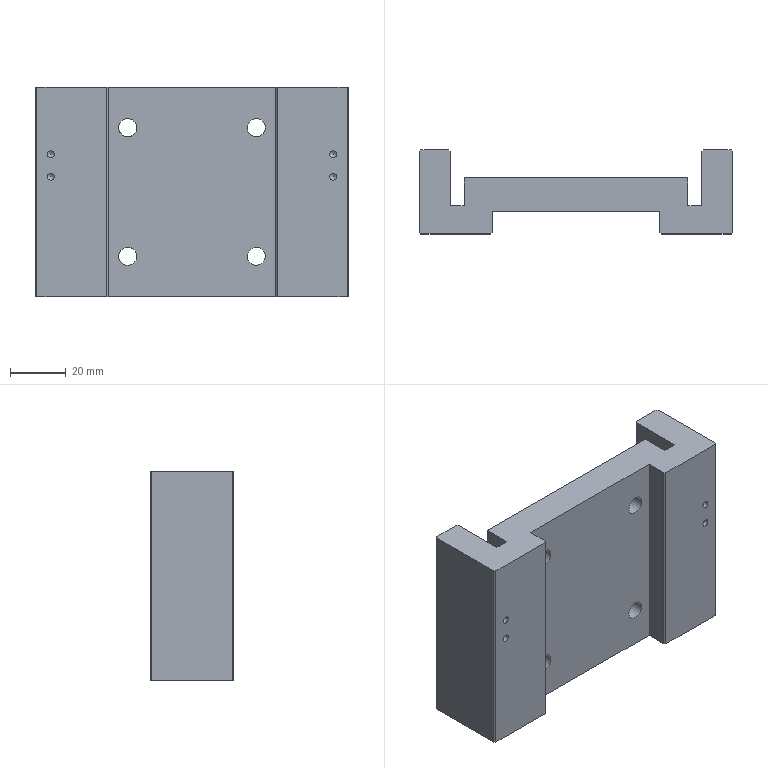Part | NX | 1 solid | 54 faces | box 112 x 30 x 75 mm | volume 135942 mm3 | plane 30 | cylinder 16 | cone 8 | commonest cylinder face diameters 2.5 x4 5 x4 6.5 x4 11 x4
STEP:
#1=CARTESIAN_POINT('',(-30.,-7.5,37.5));
#2=VERTEX_POINT('',#1);
#3=CARTESIAN_POINT('',(-30.,0.,37.5));
#4=VERTEX_POINT('',#3);
#5=CARTESIAN_POINT('',(-30.,0.,37.5));
#6=DIRECTION('',(0.,1.,0.));
#7=VECTOR('',#6,1000.);
#8=LINE('',#5,#7);
#9=EDGE_CURVE('',#2,#4,#8,.T.);
#10=ORIENTED_EDGE('',*,*,#9,.F.);
#11=CARTESIAN_POINT('',(-30.,-7.5,-37.5));
#12=VERTEX_POINT('',#11);
#13=CARTESIAN_POINT('',(-30.,-7.5,37.5));
#14=DIRECTION('',(0.,0.,-1.));
#15=VECTOR('',#14,1000.);
#16=LINE('',#13,#15);
#17=EDGE_CURVE('',#2,#12,#16,.T.);
#18=ORIENTED_EDGE('',*,*,#17,.T.);
#19=CARTESIAN_POINT('',(-30.,0.,-37.5));
#20=VERTEX_POINT('',#19);
#21=CARTESIAN_POINT('',(-30.,0.,-37.5));
#22=DIRECTION('',(0.,1.,0.));
#23=VECTOR('',#22,1000.);
#24=LINE('',#21,#23);
#25=EDGE_CURVE('',#12,#20,#24,.T.);
#26=ORIENTED_EDGE('',*,*,#25,.T.);
#27=CARTESIAN_POINT('',(-30.,0.,37.5));
#28=DIRECTION('',(0.,0.,-1.));
#29=VECTOR('',#28,1000.);
#30=LINE('',#27,#29);
#31=EDGE_CURVE('',#4,#20,#30,.T.);
#32=ORIENTED_EDGE('',*,*,#31,.F.);
#33=EDGE_LOOP('',(#10,#18,#26,#32));
#34=FACE_BOUND('',#33,.T.);
#35=CARTESIAN_POINT('',(-30.,0.,37.5));
#36=DIRECTION('',(-1.,0.,0.));
#37=DIRECTION('',(0.,-1.,0.));
#38=AXIS2_PLACEMENT_3D('',#35,#36,#37);
#39=PLANE('',#38);
#40=ADVANCED_FACE('',(#34),#39,.F.);
#41=CARTESIAN_POINT('',(-26.25,0.,-23.));
#42=VERTEX_POINT('',#41);
#43=CARTESIAN_POINT('',(-23.,0.,-23.));
#44=DIRECTION('',(0.,1.,0.));
#45=DIRECTION('',(-1.,0.,0.));
#46=AXIS2_PLACEMENT_3D('',#43,#44,#45);
#47=CIRCLE('',#46,3.25);
#48=EDGE_CURVE('',#42,#42,#47,.T.);
#49=ORIENTED_EDGE('',*,*,#48,.T.);
#50=EDGE_LOOP('',(#49));
#51=FACE_BOUND('',#50,.T.);
#52=CARTESIAN_POINT('',(-26.25,0.,23.));
#53=VERTEX_POINT('',#52);
#54=CARTESIAN_POINT('',(-23.,0.,23.));
#55=DIRECTION('',(0.,1.,0.));
#56=DIRECTION('',(-1.,0.,0.));
#57=AXIS2_PLACEMENT_3D('',#54,#55,#56);
#58=CIRCLE('',#57,3.25);
#59=EDGE_CURVE('',#53,#53,#58,.T.);
#60=ORIENTED_EDGE('',*,*,#59,.T.);
#61=EDGE_LOOP('',(#60));
#62=FACE_BOUND('',#61,.T.);
#63=CARTESIAN_POINT('',(19.75,0.,23.));
#64=VERTEX_POINT('',#63);
#65=CARTESIAN_POINT('',(23.,0.,23.));
#66=DIRECTION('',(0.,1.,0.));
#67=DIRECTION('',(-1.,0.,0.));
#68=AXIS2_PLACEMENT_3D('',#65,#66,#67);
#69=CIRCLE('',#68,3.25);
#70=EDGE_CURVE('',#64,#64,#69,.T.);
#71=ORIENTED_EDGE('',*,*,#70,.T.);
#72=EDGE_LOOP('',(#71));
#73=FACE_BOUND('',#72,.T.);
#74=CARTESIAN_POINT('',(19.75,0.,-23.));
#75=VERTEX_POINT('',#74);
#76=CARTESIAN_POINT('',(23.,0.,-23.));
#77=DIRECTION('',(0.,1.,0.));
#78=DIRECTION('',(-1.,0.,0.));
#79=AXIS2_PLACEMENT_3D('',#76,#77,#78);
#80=CIRCLE('',#79,3.25);
#81=EDGE_CURVE('',#75,#75,#80,.T.);
#82=ORIENTED_EDGE('',*,*,#81,.T.);
#83=EDGE_LOOP('',(#82));
#84=FACE_BOUND('',#83,.T.);
#85=CARTESIAN_POINT('',(30.,0.,-37.5));
#86=VERTEX_POINT('',#85);
#87=CARTESIAN_POINT('',(30.,0.,-37.5));
#88=DIRECTION('',(1.,0.,0.));
#89=VECTOR('',#88,1000.);
#90=LINE('',#87,#89);
#91=EDGE_CURVE('',#20,#86,#90,.T.);
#92=ORIENTED_EDGE('',*,*,#91,.T.);
#93=CARTESIAN_POINT('',(30.,0.,37.5));
#94=VERTEX_POINT('',#93);
#95=CARTESIAN_POINT('',(30.,0.,37.5));
#96=DIRECTION('',(0.,0.,-1.));
#97=VECTOR('',#96,1000.);
#98=LINE('',#95,#97);
#99=EDGE_CURVE('',#94,#86,#98,.T.);
#100=ORIENTED_EDGE('',*,*,#99,.F.);
#101=CARTESIAN_POINT('',(30.,0.,37.5));
#102=DIRECTION('',(1.,0.,0.));
#103=VECTOR('',#102,1000.);
#104=LINE('',#101,#103);
#105=EDGE_CURVE('',#4,#94,#104,.T.);
#106=ORIENTED_EDGE('',*,*,#105,.F.);
#107=ORIENTED_EDGE('',*,*,#31,.T.);
#108=EDGE_LOOP('',(#92,#100,#106,#107));
#109=FACE_BOUND('',#108,.T.);
#110=CARTESIAN_POINT('',(30.,0.,37.5));
#111=DIRECTION('',(0.,1.,0.));
#112=DIRECTION('',(-1.,0.,0.));
#113=AXIS2_PLACEMENT_3D('',#110,#111,#112);
#114=PLANE('',#113);
#115=ADVANCED_FACE('',(#51,#62,#73,#84,#109),#114,.F.);
#116=CARTESIAN_POINT('',(30.,-7.5,-37.5));
#117=VERTEX_POINT('',#116);
#118=CARTESIAN_POINT('',(30.,0.,-37.5));
#119=DIRECTION('',(0.,-1.,0.));
#120=VECTOR('',#119,1000.);
#121=LINE('',#118,#120);
#122=EDGE_CURVE('',#86,#117,#121,.T.);
#123=ORIENTED_EDGE('',*,*,#122,.T.);
#124=CARTESIAN_POINT('',(30.,-7.5,37.5));
#125=VERTEX_POINT('',#124);
#126=CARTESIAN_POINT('',(30.,-7.5,37.5));
#127=DIRECTION('',(0.,0.,1.));
#128=VECTOR('',#127,1000.);
#129=LINE('',#126,#128);
#130=EDGE_CURVE('',#117,#125,#129,.T.);
#131=ORIENTED_EDGE('',*,*,#130,.T.);
#132=CARTESIAN_POINT('',(30.,0.,37.5));
#133=DIRECTION('',(0.,-1.,0.));
#134=VECTOR('',#133,1000.);
#135=LINE('',#132,#134);
#136=EDGE_CURVE('',#94,#125,#135,.T.);
#137=ORIENTED_EDGE('',*,*,#136,.F.);
#138=ORIENTED_EDGE('',*,*,#99,.T.);
#139=EDGE_LOOP('',(#123,#131,#137,#138));
#140=FACE_BOUND('',#139,.T.);
#141=CARTESIAN_POINT('',(30.,0.,37.5));
#142=DIRECTION('',(1.,0.,0.));
#143=DIRECTION('',(0.,0.,-1.));
#144=AXIS2_PLACEMENT_3D('',#141,#142,#143);
#145=PLANE('',#144);
#146=ADVANCED_FACE('',(#140),#145,.F.);
#147=CARTESIAN_POINT('',(50.5,-8.,12.25));
#148=VERTEX_POINT('',#147);
#149=CARTESIAN_POINT('',(50.5,-8.,13.5));
#150=DIRECTION('',(0.,-1.,0.));
#151=DIRECTION('',(0.,0.,-1.));
#152=AXIS2_PLACEMENT_3D('',#149,#150,#151);
#153=CIRCLE('',#152,1.25);
#154=EDGE_CURVE('',#148,#148,#153,.T.);
#155=ORIENTED_EDGE('',*,*,#154,.F.);
#156=EDGE_LOOP('',(#155));
#157=FACE_BOUND('',#156,.T.);
#158=CARTESIAN_POINT('',(50.5,-8.,4.25));
#159=VERTEX_POINT('',#158);
#160=CARTESIAN_POINT('',(50.5,-8.,5.5));
#161=DIRECTION('',(0.,-1.,0.));
#162=DIRECTION('',(0.,0.,-1.));
#163=AXIS2_PLACEMENT_3D('',#160,#161,#162);
#164=CIRCLE('',#163,1.25);
#165=EDGE_CURVE('',#159,#159,#164,.T.);
#166=ORIENTED_EDGE('',*,*,#165,.F.);
#167=EDGE_LOOP('',(#166));
#168=FACE_BOUND('',#167,.T.);
#169=CARTESIAN_POINT('',(30.5,-8.,-37.5));
#170=VERTEX_POINT('',#169);
#171=CARTESIAN_POINT('',(55.5,-8.,-37.5));
#172=VERTEX_POINT('',#171);
#173=CARTESIAN_POINT('',(30.,-8.,-37.5));
#174=DIRECTION('',(1.,0.,0.));
#175=VECTOR('',#174,1000.);
#176=LINE('',#173,#175);
#177=EDGE_CURVE('',#170,#172,#176,.T.);
#178=ORIENTED_EDGE('',*,*,#177,.T.);
#179=CARTESIAN_POINT('',(55.5,-8.,37.5));
#180=VERTEX_POINT('',#179);
#181=CARTESIAN_POINT('',(55.5,-8.,37.5));
#182=DIRECTION('',(0.,0.,1.));
#183=VECTOR('',#182,1000.);
#184=LINE('',#181,#183);
#185=EDGE_CURVE('',#172,#180,#184,.T.);
#186=ORIENTED_EDGE('',*,*,#185,.T.);
#187=CARTESIAN_POINT('',(30.5,-8.,37.5));
#188=VERTEX_POINT('',#187);
#189=CARTESIAN_POINT('',(30.,-8.,37.5));
#190=DIRECTION('',(1.,0.,0.));
#191=VECTOR('',#190,1000.);
#192=LINE('',#189,#191);
#193=EDGE_CURVE('',#188,#180,#192,.T.);
#194=ORIENTED_EDGE('',*,*,#193,.F.);
#195=CARTESIAN_POINT('',(30.5,-8.,37.5));
#196=DIRECTION('',(0.,0.,-1.));
#197=VECTOR('',#196,1000.);
#198=LINE('',#195,#197);
#199=EDGE_CURVE('',#188,#170,#198,.T.);
#200=ORIENTED_EDGE('',*,*,#199,.T.);
#201=EDGE_LOOP('',(#178,#186,#194,#200));
#202=FACE_BOUND('',#201,.T.);
#203=CARTESIAN_POINT('',(30.,-8.,37.5));
#204=DIRECTION('',(0.,1.,0.));
#205=DIRECTION('',(-1.,0.,0.));
#206=AXIS2_PLACEMENT_3D('',#203,#204,#205);
#207=PLANE('',#206);
#208=ADVANCED_FACE('',(#157,#168,#202),#207,.F.);
#209=CARTESIAN_POINT('',(56.,-7.5,-37.5));
#210=VERTEX_POINT('',#209);
#211=CARTESIAN_POINT('',(56.,21.5,-37.5));
#212=VERTEX_POINT('',#211);
#213=CARTESIAN_POINT('',(56.,-8.,-37.5));
#214=DIRECTION('',(0.,1.,0.));
#215=VECTOR('',#214,1000.);
#216=LINE('',#213,#215);
#217=EDGE_CURVE('',#210,#212,#216,.T.);
#218=ORIENTED_EDGE('',*,*,#217,.T.);
#219=CARTESIAN_POINT('',(56.,21.5,37.5));
#220=VERTEX_POINT('',#219);
#221=CARTESIAN_POINT('',(56.,21.5,37.5));
#222=DIRECTION('',(0.,0.,1.));
#223=VECTOR('',#222,1000.);
#224=LINE('',#221,#223);
#225=EDGE_CURVE('',#212,#220,#224,.T.);
#226=ORIENTED_EDGE('',*,*,#225,.T.);
#227=CARTESIAN_POINT('',(56.,-7.5,37.5));
#228=VERTEX_POINT('',#227);
#229=CARTESIAN_POINT('',(56.,-8.,37.5));
#230=DIRECTION('',(0.,1.,0.));
#231=VECTOR('',#230,1000.);
#232=LINE('',#229,#231);
#233=EDGE_CURVE('',#228,#220,#232,.T.);
#234=ORIENTED_EDGE('',*,*,#233,.F.);
#235=CARTESIAN_POINT('',(56.,-7.5,37.5));
#236=DIRECTION('',(0.,0.,-1.));
#237=VECTOR('',#236,1000.);
#238=LINE('',#235,#237);
#239=EDGE_CURVE('',#228,#210,#238,.T.);
#240=ORIENTED_EDGE('',*,*,#239,.T.);
#241=EDGE_LOOP('',(#218,#226,#234,#240));
#242=FACE_BOUND('',#241,.T.);
#243=CARTESIAN_POINT('',(56.,-8.,37.5));
#244=DIRECTION('',(-1.,0.,0.));
#245=DIRECTION('',(0.,-1.,0.));
#246=AXIS2_PLACEMENT_3D('',#243,#244,#245);
#247=PLANE('',#246);
#248=ADVANCED_FACE('',(#242),#247,.F.);
#249=CARTESIAN_POINT('',(50.,22.,-20.5));
#250=VERTEX_POINT('',#249);
#251=CARTESIAN_POINT('',(50.,22.,-23.));
#252=DIRECTION('',(0.,1.,0.));
#253=DIRECTION('',(0.,0.,1.));
#254=AXIS2_PLACEMENT_3D('',#251,#252,#253);
#255=CIRCLE('',#254,2.5);
#256=EDGE_CURVE('',#250,#250,#255,.T.);
#257=ORIENTED_EDGE('',*,*,#256,.F.);
#258=EDGE_LOOP('',(#257));
#259=FACE_BOUND('',#258,.T.);
#260=CARTESIAN_POINT('',(50.,22.,25.5));
#261=VERTEX_POINT('',#260);
#262=CARTESIAN_POINT('',(50.,22.,23.));
#263=DIRECTION('',(0.,1.,0.));
#264=DIRECTION('',(0.,0.,1.));
#265=AXIS2_PLACEMENT_3D('',#262,#263,#264);
#266=CIRCLE('',#265,2.5);
#267=EDGE_CURVE('',#261,#261,#266,.T.);
#268=ORIENTED_EDGE('',*,*,#267,.F.);
#269=EDGE_LOOP('',(#268));
#270=FACE_BOUND('',#269,.T.);
#271=CARTESIAN_POINT('',(55.5,22.,-37.5));
#272=VERTEX_POINT('',#271);
#273=CARTESIAN_POINT('',(45.5,22.,-37.5));
#274=VERTEX_POINT('',#273);
#275=CARTESIAN_POINT('',(56.,22.,-37.5));
#276=DIRECTION('',(-1.,0.,0.));
#277=VECTOR('',#276,1000.);
#278=LINE('',#275,#277);
#279=EDGE_CURVE('',#272,#274,#278,.T.);
#280=ORIENTED_EDGE('',*,*,#279,.T.);
#281=CARTESIAN_POINT('',(45.5,22.,37.5));
#282=VERTEX_POINT('',#281);
#283=CARTESIAN_POINT('',(45.5,22.,37.5));
#284=DIRECTION('',(0.,0.,1.));
#285=VECTOR('',#284,1000.);
#286=LINE('',#283,#285);
#287=EDGE_CURVE('',#274,#282,#286,.T.);
#288=ORIENTED_EDGE('',*,*,#287,.T.);
#289=CARTESIAN_POINT('',(55.5,22.,37.5));
#290=VERTEX_POINT('',#289);
#291=CARTESIAN_POINT('',(56.,22.,37.5));
#292=DIRECTION('',(-1.,0.,0.));
#293=VECTOR('',#292,1000.);
#294=LINE('',#291,#293);
#295=EDGE_CURVE('',#290,#282,#294,.T.);
#296=ORIENTED_EDGE('',*,*,#295,.F.);
#297=CARTESIAN_POINT('',(55.5,22.,37.5));
#298=DIRECTION('',(0.,0.,-1.));
#299=VECTOR('',#298,1000.);
#300=LINE('',#297,#299);
#301=EDGE_CURVE('',#290,#272,#300,.T.);
#302=ORIENTED_EDGE('',*,*,#301,.T.);
#303=EDGE_LOOP('',(#280,#288,#296,#302));
#304=FACE_BOUND('',#303,.T.);
#305=CARTESIAN_POINT('',(56.,22.,37.5));
#306=DIRECTION('',(0.,-1.,0.));
#307=DIRECTION('',(0.,0.,-1.));
#308=AXIS2_PLACEMENT_3D('',#305,#306,#307);
#309=PLANE('',#308);
#310=ADVANCED_FACE('',(#259,#270,#304),#309,.F.);
#311=CARTESIAN_POINT('',(45.,21.5,37.5));
#312=VERTEX_POINT('',#311);
#313=CARTESIAN_POINT('',(45.,2.,37.5));
#314=VERTEX_POINT('',#313);
#315=CARTESIAN_POINT('',(45.,22.,37.5));
#316=DIRECTION('',(0.,-1.,0.));
#317=VECTOR('',#316,1000.);
#318=LINE('',#315,#317);
#319=EDGE_CURVE('',#312,#314,#318,.T.);
#320=ORIENTED_EDGE('',*,*,#319,.F.);
#321=CARTESIAN_POINT('',(45.,21.5,-37.5));
#322=VERTEX_POINT('',#321);
#323=CARTESIAN_POINT('',(45.,21.5,37.5));
#324=DIRECTION('',(0.,0.,-1.));
#325=VECTOR('',#324,1000.);
#326=LINE('',#323,#325);
#327=EDGE_CURVE('',#312,#322,#326,.T.);
#328=ORIENTED_EDGE('',*,*,#327,.T.);
#329=CARTESIAN_POINT('',(45.,2.,-37.5));
#330=VERTEX_POINT('',#329);
#331=CARTESIAN_POINT('',(45.,22.,-37.5));
#332=DIRECTION('',(0.,-1.,0.));
#333=VECTOR('',#332,1000.);
#334=LINE('',#331,#333);
#335=EDGE_CURVE('',#322,#330,#334,.T.);
#336=ORIENTED_EDGE('',*,*,#335,.T.);
#337=CARTESIAN_POINT('',(45.,2.,37.5));
#338=DIRECTION('',(0.,0.,-1.));
#339=VECTOR('',#338,1000.);
#340=LINE('',#337,#339);
#341=EDGE_CURVE('',#314,#330,#340,.T.);
#342=ORIENTED_EDGE('',*,*,#341,.F.);
#343=EDGE_LOOP('',(#320,#328,#336,#342));
#344=FACE_BOUND('',#343,.T.);
#345=CARTESIAN_POINT('',(45.,22.,37.5));
#346=DIRECTION('',(1.,0.,0.));
#347=DIRECTION('',(0.,0.,-1.));
#348=AXIS2_PLACEMENT_3D('',#345,#346,#347);
#349=PLANE('',#348);
#350=ADVANCED_FACE('',(#344),#349,.F.);
#351=CARTESIAN_POINT('',(-23.,12.,-17.5));
#352=VERTEX_POINT('',#351);
#353=CARTESIAN_POINT('',(-23.,12.,-23.));
#354=DIRECTION('',(0.,1.,0.));
#355=DIRECTION('',(0.,0.,1.));
#356=AXIS2_PLACEMENT_3D('',#353,#354,#355);
#357=CIRCLE('',#356,5.5);
#358=EDGE_CURVE('',#352,#352,#357,.T.);
#359=ORIENTED_EDGE('',*,*,#358,.F.);
#360=EDGE_LOOP('',(#359));
#361=FACE_BOUND('',#360,.T.);
#362=CARTESIAN_POINT('',(-23.,12.,28.5));
#363=VERTEX_POINT('',#362);
#364=CARTESIAN_POINT('',(-23.,12.,23.));
#365=DIRECTION('',(0.,1.,0.));
#366=DIRECTION('',(0.,0.,1.));
#367=AXIS2_PLACEMENT_3D('',#364,#365,#366);
#368=CIRCLE('',#367,5.5);
#369=EDGE_CURVE('',#363,#363,#368,.T.);
#370=ORIENTED_EDGE('',*,*,#369,.F.);
#371=EDGE_LOOP('',(#370));
#372=FACE_BOUND('',#371,.T.);
#373=CARTESIAN_POINT('',(23.,12.,28.5));
#374=VERTEX_POINT('',#373);
#375=CARTESIAN_POINT('',(23.,12.,23.));
#376=DIRECTION('',(0.,1.,0.));
#377=DIRECTION('',(0.,0.,1.));
#378=AXIS2_PLACEMENT_3D('',#375,#376,#377);
#379=CIRCLE('',#378,5.5);
#380=EDGE_CURVE('',#374,#374,#379,.T.);
#381=ORIENTED_EDGE('',*,*,#380,.F.);
#382=EDGE_LOOP('',(#381));
#383=FACE_BOUND('',#382,.T.);
#384=CARTESIAN_POINT('',(23.,12.,-17.5));
#385=VERTEX_POINT('',#384);
#386=CARTESIAN_POINT('',(23.,12.,-23.));
#387=DIRECTION('',(0.,1.,0.));
#388=DIRECTION('',(0.,0.,1.));
#389=AXIS2_PLACEMENT_3D('',#386,#387,#388);
#390=CIRCLE('',#389,5.5);
#391=EDGE_CURVE('',#385,#385,#390,.T.);
#392=ORIENTED_EDGE('',*,*,#391,.F.);
#393=EDGE_LOOP('',(#392));
#394=FACE_BOUND('',#393,.T.);
#395=CARTESIAN_POINT('',(40.,12.,-37.5));
#396=VERTEX_POINT('',#395);
#397=CARTESIAN_POINT('',(-40.,12.,-37.5));
#398=VERTEX_POINT('',#397);
#399=CARTESIAN_POINT('',(-45.,12.,-37.5));
#400=DIRECTION('',(-1.,0.,0.));
#401=VECTOR('',#400,1000.);
#402=LINE('',#399,#401);
#403=EDGE_CURVE('',#396,#398,#402,.T.);
#404=ORIENTED_EDGE('',*,*,#403,.T.);
#405=CARTESIAN_POINT('',(-40.,12.,37.5));
#406=VERTEX_POINT('',#405);
#407=CARTESIAN_POINT('',(-40.,12.,37.5));
#408=DIRECTION('',(0.,0.,-1.));
#409=VECTOR('',#408,1000.);
#410=LINE('',#407,#409);
#411=EDGE_CURVE('',#406,#398,#410,.T.);
#412=ORIENTED_EDGE('',*,*,#411,.F.);
#413=CARTESIAN_POINT('',(40.,12.,37.5));
#414=VERTEX_POINT('',#413);
#415=CARTESIAN_POINT('',(-45.,12.,37.5));
#416=DIRECTION('',(-1.,0.,0.));
#417=VECTOR('',#416,1000.);
#418=LINE('',#415,#417);
#419=EDGE_CURVE('',#414,#406,#418,.T.);
#420=ORIENTED_EDGE('',*,*,#419,.F.);
#421=CARTESIAN_POINT('',(40.,12.,37.5));
#422=DIRECTION('',(0.,0.,-1.));
#423=VECTOR('',#422,1000.);
#424=LINE('',#421,#423);
#425=EDGE_CURVE('',#414,#396,#424,.T.);
#426=ORIENTED_EDGE('',*,*,#425,.T.);
#427=EDGE_LOOP('',(#404,#412,#420,#426));
#428=FACE_BOUND('',#427,.T.);
#429=CARTESIAN_POINT('',(-45.,12.,37.5));
#430=DIRECTION('',(0.,-1.,0.));
#431=DIRECTION('',(1.,0.,0.));
#432=AXIS2_PLACEMENT_3D('',#429,#430,#431);
#433=PLANE('',#432);
#434=ADVANCED_FACE('',(#361,#372,#383,#394,#428),#433,.F.);
#435=CARTESIAN_POINT('',(-45.,2.,-37.5));
#436=VERTEX_POINT('',#435);
#437=CARTESIAN_POINT('',(-45.,21.5,-37.5));
#438=VERTEX_POINT('',#437);
#439=CARTESIAN_POINT('',(-45.,22.,-37.5));
#440=DIRECTION('',(0.,1.,0.));
#441=VECTOR('',#440,1000.);
#442=LINE('',#439,#441);
#443=EDGE_CURVE('',#436,#438,#442,.T.);
#444=ORIENTED_EDGE('',*,*,#443,.T.);
#445=CARTESIAN_POINT('',(-45.,21.5,37.5));
#446=VERTEX_POINT('',#445);
#447=CARTESIAN_POINT('',(-45.,21.5,37.5));
#448=DIRECTION('',(0.,0.,1.));
#449=VECTOR('',#448,1000.);
#450=LINE('',#447,#449);
#451=EDGE_CURVE('',#438,#446,#450,.T.);
#452=ORIENTED_EDGE('',*,*,#451,.T.);
#453=CARTESIAN_POINT('',(-45.,2.,37.5));
#454=VERTEX_POINT('',#453);
#455=CARTESIAN_POINT('',(-45.,22.,37.5));
#456=DIRECTION('',(0.,1.,0.));
#457=VECTOR('',#456,1000.);
#458=LINE('',#455,#457);
#459=EDGE_CURVE('',#454,#446,#458,.T.);
#460=ORIENTED_EDGE('',*,*,#459,.F.);
#461=CARTESIAN_POINT('',(-45.,2.,37.5));
#462=DIRECTION('',(0.,0.,-1.));
#463=VECTOR('',#462,1000.);
#464=LINE('',#461,#463);
#465=EDGE_CURVE('',#454,#436,#464,.T.);
#466=ORIENTED_EDGE('',*,*,#465,.T.);
#467=EDGE_LOOP('',(#444,#452,#460,#466));
#468=FACE_BOUND('',#467,.T.);
#469=CARTESIAN_POINT('',(-45.,22.,37.5));
#470=DIRECTION('',(-1.,0.,0.));
#471=DIRECTION('',(0.,0.,1.));
#472=AXIS2_PLACEMENT_3D('',#469,#470,#471);
#473=PLANE('',#472);
#474=ADVANCED_FACE('',(#468),#473,.F.);
#475=CARTESIAN_POINT('',(-50.,22.,-20.5));
#476=VERTEX_POINT('',#475);
#477=CARTESIAN_POINT('',(-50.,22.,-23.));
#478=DIRECTION('',(0.,1.,0.));
#479=DIRECTION('',(0.,0.,1.));
#480=AXIS2_PLACEMENT_3D('',#477,#478,#479);
#481=CIRCLE('',#480,2.5);
#482=EDGE_CURVE('',#476,#476,#481,.T.);
#483=ORIENTED_EDGE('',*,*,#482,.F.);
#484=EDGE_LOOP('',(#483));
#485=FACE_BOUND('',#484,.T.);
#486=CARTESIAN_POINT('',(-50.,22.,25.5));
#487=VERTEX_POINT('',#486);
#488=CARTESIAN_POINT('',(-50.,22.,23.));
#489=DIRECTION('',(0.,1.,0.));
#490=DIRECTION('',(0.,0.,1.));
#491=AXIS2_PLACEMENT_3D('',#488,#489,#490);
#492=CIRCLE('',#491,2.5);
#493=EDGE_CURVE('',#487,#487,#492,.T.);
#494=ORIENTED_EDGE('',*,*,#493,.F.);
#495=EDGE_LOOP('',(#494));
#496=FACE_BOUND('',#495,.T.);
#497=CARTESIAN_POINT('',(-45.5,22.,-37.5));
#498=VERTEX_POINT('',#497);
#499=CARTESIAN_POINT('',(-55.5,22.,-37.5));
#500=VERTEX_POINT('',#499);
#501=CARTESIAN_POINT('',(-56.,22.,-37.5));
#502=DIRECTION('',(-1.,0.,0.));
#503=VECTOR('',#502,1000.);
#504=LINE('',#501,#503);
#505=EDGE_CURVE('',#498,#500,#504,.T.);
#506=ORIENTED_EDGE('',*,*,#505,.T.);
#507=CARTESIAN_POINT('',(-55.5,22.,37.5));
#508=VERTEX_POINT('',#507);
#509=CARTESIAN_POINT('',(-55.5,22.,37.5));
#510=DIRECTION('',(0.,0.,1.));
#511=VECTOR('',#510,1000.);
#512=LINE('',#509,#511);
#513=EDGE_CURVE('',#500,#508,#512,.T.);
#514=ORIENTED_EDGE('',*,*,#513,.T.);
#515=CARTESIAN_POINT('',(-45.5,22.,37.5));
#516=VERTEX_POINT('',#515);
#517=CARTESIAN_POINT('',(-56.,22.,37.5));
#518=DIRECTION('',(-1.,0.,0.));
#519=VECTOR('',#518,1000.);
#520=LINE('',#517,#519);
#521=EDGE_CURVE('',#516,#508,#520,.T.);
#522=ORIENTED_EDGE('',*,*,#521,.F.);
#523=CARTESIAN_POINT('',(-45.5,22.,37.5));
#524=DIRECTION('',(0.,0.,-1.));
#525=VECTOR('',#524,1000.);
#526=LINE('',#523,#525);
#527=EDGE_CURVE('',#516,#498,#526,.T.);
#528=ORIENTED_EDGE('',*,*,#527,.T.);
#529=EDGE_LOOP('',(#506,#514,#522,#528));
#530=FACE_BOUND('',#529,.T.);
#531=CARTESIAN_POINT('',(-56.,22.,37.5));
#532=DIRECTION('',(0.,-1.,0.));
#533=DIRECTION('',(1.,0.,0.));
#534=AXIS2_PLACEMENT_3D('',#531,#532,#533);
#535=PLANE('',#534);
#536=ADVANCED_FACE('',(#485,#496,#530),#535,.F.);
#537=CARTESIAN_POINT('',(-56.,21.5,37.5));
#538=VERTEX_POINT('',#537);
#539=CARTESIAN_POINT('',(-56.,-7.5,37.5));
#540=VERTEX_POINT('',#539);
#541=CARTESIAN_POINT('',(-56.,-8.,37.5));
#542=DIRECTION('',(0.,-1.,0.));
#543=VECTOR('',#542,1000.);
#544=LINE('',#541,#543);
#545=EDGE_CURVE('',#538,#540,#544,.T.);
#546=ORIENTED_EDGE('',*,*,#545,.F.);
#547=CARTESIAN_POINT('',(-56.,21.5,-37.5));
#548=VERTEX_POINT('',#547);
#549=CARTESIAN_POINT('',(-56.,21.5,37.5));
#550=DIRECTION('',(0.,0.,-1.));
#551=VECTOR('',#550,1000.);
#552=LINE('',#549,#551);
#553=EDGE_CURVE('',#538,#548,#552,.T.);
#554=ORIENTED_EDGE('',*,*,#553,.T.);
#555=CARTESIAN_POINT('',(-56.,-7.5,-37.5));
#556=VERTEX_POINT('',#555);
#557=CARTESIAN_POINT('',(-56.,-8.,-37.5));
#558=DIRECTION('',(0.,-1.,0.));
#559=VECTOR('',#558,1000.);
#560=LINE('',#557,#559);
#561=EDGE_CURVE('',#548,#556,#560,.T.);
#562=ORIENTED_EDGE('',*,*,#561,.T.);
#563=CARTESIAN_POINT('',(-56.,-7.5,37.5));
#564=DIRECTION('',(0.,0.,1.));
#565=VECTOR('',#564,1000.);
#566=LINE('',#563,#565);
#567=EDGE_CURVE('',#556,#540,#566,.T.);
#568=ORIENTED_EDGE('',*,*,#567,.T.);
#569=EDGE_LOOP('',(#546,#554,#562,#568));
#570=FACE_BOUND('',#569,.T.);
#571=CARTESIAN_POINT('',(-56.,-8.,37.5));
#572=DIRECTION('',(1.,0.,0.));
#573=DIRECTION('',(0.,1.,0.));
#574=AXIS2_PLACEMENT_3D('',#571,#572,#573);
#575=PLANE('',#574);
#576=ADVANCED_FACE('',(#570),#575,.F.);
#577=CARTESIAN_POINT('',(-50.5,-8.,12.25));
#578=VERTEX_POINT('',#577);
#579=CARTESIAN_POINT('',(-50.5,-8.,13.5));
#580=DIRECTION('',(0.,-1.,0.));
#581=DIRECTION('',(0.,0.,-1.));
#582=AXIS2_PLACEMENT_3D('',#579,#580,#581);
#583=CIRCLE('',#582,1.25);
#584=EDGE_CURVE('',#578,#578,#583,.T.);
#585=ORIENTED_EDGE('',*,*,#584,.F.);
#586=EDGE_LOOP('',(#585));
#587=FACE_BOUND('',#586,.T.);
#588=CARTESIAN_POINT('',(-50.5,-8.,4.25));
#589=VERTEX_POINT('',#588);
#590=CARTESIAN_POINT('',(-50.5,-8.,5.5));
#591=DIRECTION('',(0.,-1.,0.));
#592=DIRECTION('',(0.,0.,-1.));
#593=AXIS2_PLACEMENT_3D('',#590,#591,#592);
#594=CIRCLE('',#593,1.25);
#595=EDGE_CURVE('',#589,#589,#594,.T.);
#596=ORIENTED_EDGE('',*,*,#595,.F.);
#597=EDGE_LOOP('',(#596));
#598=FACE_BOUND('',#597,.T.);
#599=CARTESIAN_POINT('',(-55.5,-8.,-37.5));
#600=VERTEX_POINT('',#599);
#601=CARTESIAN_POINT('',(-30.5,-8.,-37.5));
#602=VERTEX_POINT('',#601);
#603=CARTESIAN_POINT('',(-30.,-8.,-37.5));
#604=DIRECTION('',(1.,0.,0.));
#605=VECTOR('',#604,1000.);
#606=LINE('',#603,#605);
#607=EDGE_CURVE('',#600,#602,#606,.T.);
#608=ORIENTED_EDGE('',*,*,#607,.T.);
#609=CARTESIAN_POINT('',(-30.5,-8.,37.5));
#610=VERTEX_POINT('',#609);
#611=CARTESIAN_POINT('',(-30.5,-8.,37.5));
#612=DIRECTION('',(0.,0.,1.));
#613=VECTOR('',#612,1000.);
#614=LINE('',#611,#613);
#615=EDGE_CURVE('',#602,#610,#614,.T.);
#616=ORIENTED_EDGE('',*,*,#615,.T.);
#617=CARTESIAN_POINT('',(-55.5,-8.,37.5));
#618=VERTEX_POINT('',#617);
#619=CARTESIAN_POINT('',(-30.,-8.,37.5));
#620=DIRECTION('',(1.,0.,0.));
#621=VECTOR('',#620,1000.);
#622=LINE('',#619,#621);
#623=EDGE_CURVE('',#618,#610,#622,.T.);
#624=ORIENTED_EDGE('',*,*,#623,.F.);
#625=CARTESIAN_POINT('',(-55.5,-8.,37.5));
#626=DIRECTION('',(0.,0.,-1.));
#627=VECTOR('',#626,1000.);
#628=LINE('',#625,#627);
#629=EDGE_CURVE('',#618,#600,#628,.T.);
#630=ORIENTED_EDGE('',*,*,#629,.T.);
#631=EDGE_LOOP('',(#608,#616,#624,#630));
#632=FACE_BOUND('',#631,.T.);
#633=CARTESIAN_POINT('',(-30.,-8.,37.5));
#634=DIRECTION('',(0.,1.,0.));
#635=DIRECTION('',(-1.,0.,0.));
#636=AXIS2_PLACEMENT_3D('',#633,#634,#635);
#637=PLANE('',#636);
#638=ADVANCED_FACE('',(#587,#598,#632),#637,.F.);
#639=CARTESIAN_POINT('',(-40.,2.,37.5));
#640=VERTEX_POINT('',#639);
#641=CARTESIAN_POINT('',(-45.,2.,37.5));
#642=DIRECTION('',(-1.,0.,0.));
#643=VECTOR('',#642,1000.);
#644=LINE('',#641,#643);
#645=EDGE_CURVE('',#640,#454,#644,.T.);
#646=ORIENTED_EDGE('',*,*,#645,.T.);
#647=ORIENTED_EDGE('',*,*,#459,.T.);
#648=CARTESIAN_POINT('',(-45.5,22.,37.5));
#649=DIRECTION('',(0.7071,-0.7071,0.));
#650=VECTOR('',#649,1000.);
#651=LINE('',#648,#650);
#652=EDGE_CURVE('',#446,#516,#651,.F.);
#653=ORIENTED_EDGE('',*,*,#652,.T.);
#654=ORIENTED_EDGE('',*,*,#521,.T.);
#655=CARTESIAN_POINT('',(-56.,21.5,37.5));
#656=DIRECTION('',(0.7071,0.7071,0.));
#657=VECTOR('',#656,1000.);
#658=LINE('',#655,#657);
#659=EDGE_CURVE('',#508,#538,#658,.F.);
#660=ORIENTED_EDGE('',*,*,#659,.T.);
#661=ORIENTED_EDGE('',*,*,#545,.T.);
#662=CARTESIAN_POINT('',(-55.5,-8.,37.5));
#663=DIRECTION('',(-0.7071,0.7071,0.));
#664=VECTOR('',#663,1000.);
#665=LINE('',#662,#664);
#666=EDGE_CURVE('',#540,#618,#665,.F.);
#667=ORIENTED_EDGE('',*,*,#666,.T.);
#668=ORIENTED_EDGE('',*,*,#623,.T.);
#669=CARTESIAN_POINT('',(-30.,-7.5,37.5));
#670=DIRECTION('',(-0.7071,-0.7071,0.));
#671=VECTOR('',#670,1000.);
#672=LINE('',#669,#671);
#673=EDGE_CURVE('',#610,#2,#672,.F.);
#674=ORIENTED_EDGE('',*,*,#673,.T.);
#675=ORIENTED_EDGE('',*,*,#9,.T.);
#676=ORIENTED_EDGE('',*,*,#105,.T.);
#677=ORIENTED_EDGE('',*,*,#136,.T.);
#678=CARTESIAN_POINT('',(30.5,-8.,37.5));
#679=DIRECTION('',(-0.7071,0.7071,0.));
#680=VECTOR('',#679,1000.);
#681=LINE('',#678,#680);
#682=EDGE_CURVE('',#125,#188,#681,.F.);
#683=ORIENTED_EDGE('',*,*,#682,.T.);
#684=ORIENTED_EDGE('',*,*,#193,.T.);
#685=CARTESIAN_POINT('',(56.,-7.5,37.5));
#686=DIRECTION('',(-0.7071,-0.7071,0.));
#687=VECTOR('',#686,1000.);
#688=LINE('',#685,#687);
#689=EDGE_CURVE('',#180,#228,#688,.F.);
#690=ORIENTED_EDGE('',*,*,#689,.T.);
#691=ORIENTED_EDGE('',*,*,#233,.T.);
#692=CARTESIAN_POINT('',(55.5,22.,37.5));
#693=DIRECTION('',(0.7071,-0.7071,0.));
#694=VECTOR('',#693,1000.);
#695=LINE('',#692,#694);
#696=EDGE_CURVE('',#220,#290,#695,.F.);
#697=ORIENTED_EDGE('',*,*,#696,.T.);
#698=ORIENTED_EDGE('',*,*,#295,.T.);
#699=CARTESIAN_POINT('',(45.,21.5,37.5));
#700=DIRECTION('',(0.7071,0.7071,0.));
#701=VECTOR('',#700,1000.);
#702=LINE('',#699,#701);
#703=EDGE_CURVE('',#282,#312,#702,.F.);
#704=ORIENTED_EDGE('',*,*,#703,.T.);
#705=ORIENTED_EDGE('',*,*,#319,.T.);
#706=CARTESIAN_POINT('',(40.,2.,37.5));
#707=VERTEX_POINT('',#706);
#708=CARTESIAN_POINT('',(45.,2.,37.5));
#709=DIRECTION('',(-1.,0.,0.));
#710=VECTOR('',#709,1000.);
#711=LINE('',#708,#710);
#712=EDGE_CURVE('',#314,#707,#711,.T.);
#713=ORIENTED_EDGE('',*,*,#712,.T.);
#714=CARTESIAN_POINT('',(40.,12.,37.5));
#715=DIRECTION('',(0.,1.,0.));
#716=VECTOR('',#715,1000.);
#717=LINE('',#714,#716);
#718=EDGE_CURVE('',#707,#414,#717,.T.);
#719=ORIENTED_EDGE('',*,*,#718,.T.);
#720=ORIENTED_EDGE('',*,*,#419,.T.);
#721=CARTESIAN_POINT('',(-40.,12.,37.5));
#722=DIRECTION('',(0.,-1.,0.));
#723=VECTOR('',#722,1000.);
#724=LINE('',#721,#723);
#725=EDGE_CURVE('',#406,#640,#724,.T.);
#726=ORIENTED_EDGE('',*,*,#725,.T.);
#727=EDGE_LOOP('',(#646,#647,#653,#654,#660,#661,#667,#668,#674,#675,#676,#677,#683,#684,#690,#691,#697,#698,#704,#705,#713,#719,#720,#726));
#728=FACE_BOUND('',#727,.T.);
#729=CARTESIAN_POINT('',(0.,0.,37.5));
#730=DIRECTION('',(0.,0.,-1.));
#731=DIRECTION('',(-1.,0.,0.));
#732=AXIS2_PLACEMENT_3D('',#729,#730,#731);
#733=PLANE('',#732);
#734=ADVANCED_FACE('',(#728),#733,.F.);
#735=ORIENTED_EDGE('',*,*,#443,.F.);
#736=CARTESIAN_POINT('',(-40.,2.,-37.5));
#737=VERTEX_POINT('',#736);
#738=CARTESIAN_POINT('',(-45.,2.,-37.5));
#739=DIRECTION('',(-1.,0.,0.));
#740=VECTOR('',#739,1000.);
#741=LINE('',#738,#740);
#742=EDGE_CURVE('',#737,#436,#741,.T.);
#743=ORIENTED_EDGE('',*,*,#742,.F.);
#744=CARTESIAN_POINT('',(-40.,12.,-37.5));
#745=DIRECTION('',(0.,-1.,0.));
#746=VECTOR('',#745,1000.);
#747=LINE('',#744,#746);
#748=EDGE_CURVE('',#398,#737,#747,.T.);
#749=ORIENTED_EDGE('',*,*,#748,.F.);
#750=ORIENTED_EDGE('',*,*,#403,.F.);
#751=CARTESIAN_POINT('',(40.,2.,-37.5));
#752=VERTEX_POINT('',#751);
#753=CARTESIAN_POINT('',(40.,12.,-37.5));
#754=DIRECTION('',(0.,1.,0.));
#755=VECTOR('',#754,1000.);
#756=LINE('',#753,#755);
#757=EDGE_CURVE('',#752,#396,#756,.T.);
#758=ORIENTED_EDGE('',*,*,#757,.F.);
#759=CARTESIAN_POINT('',(45.,2.,-37.5));
#760=DIRECTION('',(-1.,0.,0.));
#761=VECTOR('',#760,1000.);
#762=LINE('',#759,#761);
#763=EDGE_CURVE('',#330,#752,#762,.T.);
#764=ORIENTED_EDGE('',*,*,#763,.F.);
#765=ORIENTED_EDGE('',*,*,#335,.F.);
#766=CARTESIAN_POINT('',(11.75,-11.75,-37.5));
#767=DIRECTION('',(-0.7071,-0.7071,0.));
#768=VECTOR('',#767,1000.);
#769=LINE('',#766,#768);
#770=EDGE_CURVE('',#322,#274,#769,.F.);
#771=ORIENTED_EDGE('',*,*,#770,.T.);
#772=ORIENTED_EDGE('',*,*,#279,.F.);
#773=CARTESIAN_POINT('',(38.75,38.75,-37.5));
#774=DIRECTION('',(-0.7071,0.7071,0.));
#775=VECTOR('',#774,1000.);
#776=LINE('',#773,#775);
#777=EDGE_CURVE('',#272,#212,#776,.F.);
#778=ORIENTED_EDGE('',*,*,#777,.T.);
#779=ORIENTED_EDGE('',*,*,#217,.F.);
#780=CARTESIAN_POINT('',(31.75,-31.75,-37.5));
#781=DIRECTION('',(0.7071,0.7071,0.));
#782=VECTOR('',#781,1000.);
#783=LINE('',#780,#782);
#784=EDGE_CURVE('',#210,#172,#783,.F.);
#785=ORIENTED_EDGE('',*,*,#784,.T.);
#786=ORIENTED_EDGE('',*,*,#177,.F.);
#787=CARTESIAN_POINT('',(11.25,11.25,-37.5));
#788=DIRECTION('',(0.7071,-0.7071,0.));
#789=VECTOR('',#788,1000.);
#790=LINE('',#787,#789);
#791=EDGE_CURVE('',#170,#117,#790,.F.);
#792=ORIENTED_EDGE('',*,*,#791,.T.);
#793=ORIENTED_EDGE('',*,*,#122,.F.);
#794=ORIENTED_EDGE('',*,*,#91,.F.);
#795=ORIENTED_EDGE('',*,*,#25,.F.);
#796=CARTESIAN_POINT('',(-11.25,11.25,-37.5));
#797=DIRECTION('',(0.7071,0.7071,0.));
#798=VECTOR('',#797,1000.);
#799=LINE('',#796,#798);
#800=EDGE_CURVE('',#12,#602,#799,.F.);
#801=ORIENTED_EDGE('',*,*,#800,.T.);
#802=ORIENTED_EDGE('',*,*,#607,.F.);
#803=CARTESIAN_POINT('',(-31.75,-31.75,-37.5));
#804=DIRECTION('',(0.7071,-0.7071,0.));
#805=VECTOR('',#804,1000.);
#806=LINE('',#803,#805);
#807=EDGE_CURVE('',#600,#556,#806,.F.);
#808=ORIENTED_EDGE('',*,*,#807,.T.);
#809=ORIENTED_EDGE('',*,*,#561,.F.);
#810=CARTESIAN_POINT('',(-38.75,38.75,-37.5));
#811=DIRECTION('',(-0.7071,-0.7071,0.));
#812=VECTOR('',#811,1000.);
#813=LINE('',#810,#812);
#814=EDGE_CURVE('',#548,#500,#813,.F.);
#815=ORIENTED_EDGE('',*,*,#814,.T.);
#816=ORIENTED_EDGE('',*,*,#505,.F.);
#817=CARTESIAN_POINT('',(-11.75,-11.75,-37.5));
#818=DIRECTION('',(-0.7071,0.7071,0.));
#819=VECTOR('',#818,1000.);
#820=LINE('',#817,#819);
#821=EDGE_CURVE('',#498,#438,#820,.F.);
#822=ORIENTED_EDGE('',*,*,#821,.T.);
#823=EDGE_LOOP('',(#735,#743,#749,#750,#758,#764,#765,#771,#772,#778,#779,#785,#786,#792,#793,#794,#795,#801,#802,#808,#809,#815,#816,#822));
#824=FACE_BOUND('',#823,.T.);
#825=CARTESIAN_POINT('',(0.,0.,-37.5));
#826=DIRECTION('',(0.,0.,-1.));
#827=DIRECTION('',(-1.,0.,0.));
#828=AXIS2_PLACEMENT_3D('',#825,#826,#827);
#829=PLANE('',#828);
#830=ADVANCED_FACE('',(#824),#829,.T.);
#831=ORIENTED_EDGE('',*,*,#659,.F.);
#832=ORIENTED_EDGE('',*,*,#513,.F.);
#833=ORIENTED_EDGE('',*,*,#814,.F.);
#834=ORIENTED_EDGE('',*,*,#553,.F.);
#835=EDGE_LOOP('',(#831,#832,#833,#834));
#836=FACE_BOUND('',#835,.T.);
#837=CARTESIAN_POINT('',(-56.,21.5,37.5));
#838=DIRECTION('',(0.7071,-0.7071,0.));
#839=DIRECTION('',(0.,0.,-1.));
#840=AXIS2_PLACEMENT_3D('',#837,#838,#839);
#841=PLANE('',#840);
#842=ADVANCED_FACE('',(#836),#841,.F.);
#843=ORIENTED_EDGE('',*,*,#652,.F.);
#844=ORIENTED_EDGE('',*,*,#451,.F.);
#845=ORIENTED_EDGE('',*,*,#821,.F.);
#846=ORIENTED_EDGE('',*,*,#527,.F.);
#847=EDGE_LOOP('',(#843,#844,#845,#846));
#848=FACE_BOUND('',#847,.T.);
#849=CARTESIAN_POINT('',(-45.5,22.,37.5));
#850=DIRECTION('',(-0.7071,-0.7071,0.));
#851=DIRECTION('',(0.,0.,-1.));
#852=AXIS2_PLACEMENT_3D('',#849,#850,#851);
#853=PLANE('',#852);
#854=ADVANCED_FACE('',(#848),#853,.F.);
#855=ORIENTED_EDGE('',*,*,#703,.F.);
#856=ORIENTED_EDGE('',*,*,#287,.F.);
#857=ORIENTED_EDGE('',*,*,#770,.F.);
#858=ORIENTED_EDGE('',*,*,#327,.F.);
#859=EDGE_LOOP('',(#855,#856,#857,#858));
#860=FACE_BOUND('',#859,.T.);
#861=CARTESIAN_POINT('',(45.,21.5,37.5));
#862=DIRECTION('',(0.7071,-0.7071,0.));
#863=DIRECTION('',(0.,0.,-1.));
#864=AXIS2_PLACEMENT_3D('',#861,#862,#863);
#865=PLANE('',#864);
#866=ADVANCED_FACE('',(#860),#865,.F.);
#867=ORIENTED_EDGE('',*,*,#696,.F.);
#868=ORIENTED_EDGE('',*,*,#225,.F.);
#869=ORIENTED_EDGE('',*,*,#777,.F.);
#870=ORIENTED_EDGE('',*,*,#301,.F.);
#871=EDGE_LOOP('',(#867,#868,#869,#870));
#872=FACE_BOUND('',#871,.T.);
#873=CARTESIAN_POINT('',(55.5,22.,37.5));
#874=DIRECTION('',(-0.7071,-0.7071,0.));
#875=DIRECTION('',(0.,0.,-1.));
#876=AXIS2_PLACEMENT_3D('',#873,#874,#875);
#877=PLANE('',#876);
#878=ADVANCED_FACE('',(#872),#877,.F.);
#879=ORIENTED_EDGE('',*,*,#689,.F.);
#880=ORIENTED_EDGE('',*,*,#185,.F.);
#881=ORIENTED_EDGE('',*,*,#784,.F.);
#882=ORIENTED_EDGE('',*,*,#239,.F.);
#883=EDGE_LOOP('',(#879,#880,#881,#882));
#884=FACE_BOUND('',#883,.T.);
#885=CARTESIAN_POINT('',(56.,-7.5,37.5));
#886=DIRECTION('',(-0.7071,0.7071,0.));
#887=DIRECTION('',(0.,0.,-1.));
#888=AXIS2_PLACEMENT_3D('',#885,#886,#887);
#889=PLANE('',#888);
#890=ADVANCED_FACE('',(#884),#889,.F.);
#891=ORIENTED_EDGE('',*,*,#682,.F.);
#892=ORIENTED_EDGE('',*,*,#130,.F.);
#893=ORIENTED_EDGE('',*,*,#791,.F.);
#894=ORIENTED_EDGE('',*,*,#199,.F.);
#895=EDGE_LOOP('',(#891,#892,#893,#894));
#896=FACE_BOUND('',#895,.T.);
#897=CARTESIAN_POINT('',(30.5,-8.,37.5));
#898=DIRECTION('',(0.7071,0.7071,0.));
#899=DIRECTION('',(0.,0.,-1.));
#900=AXIS2_PLACEMENT_3D('',#897,#898,#899);
#901=PLANE('',#900);
#902=ADVANCED_FACE('',(#896),#901,.F.);
#903=ORIENTED_EDGE('',*,*,#673,.F.);
#904=ORIENTED_EDGE('',*,*,#615,.F.);
#905=ORIENTED_EDGE('',*,*,#800,.F.);
#906=ORIENTED_EDGE('',*,*,#17,.F.);
#907=EDGE_LOOP('',(#903,#904,#905,#906));
#908=FACE_BOUND('',#907,.T.);
#909=CARTESIAN_POINT('',(-30.,-7.5,37.5));
#910=DIRECTION('',(-0.7071,0.7071,0.));
#911=DIRECTION('',(0.,0.,-1.));
#912=AXIS2_PLACEMENT_3D('',#909,#910,#911);
#913=PLANE('',#912);
#914=ADVANCED_FACE('',(#908),#913,.F.);
#915=ORIENTED_EDGE('',*,*,#666,.F.);
#916=ORIENTED_EDGE('',*,*,#567,.F.);
#917=ORIENTED_EDGE('',*,*,#807,.F.);
#918=ORIENTED_EDGE('',*,*,#629,.F.);
#919=EDGE_LOOP('',(#915,#916,#917,#918));
#920=FACE_BOUND('',#919,.T.);
#921=CARTESIAN_POINT('',(-55.5,-8.,37.5));
#922=DIRECTION('',(0.7071,0.7071,0.));
#923=DIRECTION('',(0.,0.,-1.));
#924=AXIS2_PLACEMENT_3D('',#921,#922,#923);
#925=PLANE('',#924);
#926=ADVANCED_FACE('',(#920),#925,.F.);
#927=CARTESIAN_POINT('',(23.,5.5,-19.75));
#928=VERTEX_POINT('',#927);
#929=CARTESIAN_POINT('',(23.,5.5,-23.));
#930=DIRECTION('',(0.,1.,0.));
#931=DIRECTION('',(0.,0.,1.));
#932=AXIS2_PLACEMENT_3D('',#929,#930,#931);
#933=CIRCLE('',#932,3.25);
#934=EDGE_CURVE('',#928,#928,#933,.T.);
#935=ORIENTED_EDGE('',*,*,#934,.T.);
#936=EDGE_LOOP('',(#935));
#937=FACE_BOUND('',#936,.T.);
#938=ORIENTED_EDGE('',*,*,#81,.F.);
#939=EDGE_LOOP('',(#938));
#940=FACE_BOUND('',#939,.T.);
#941=CARTESIAN_POINT('',(23.,12.,-23.));
#942=DIRECTION('',(0.,1.,0.));
#943=DIRECTION('',(0.,0.,1.));
#944=AXIS2_PLACEMENT_3D('',#941,#942,#943);
#945=CYLINDRICAL_SURFACE('',#944,3.25);
#946=ADVANCED_FACE('',(#937,#940),#945,.F.);
#947=ORIENTED_EDGE('',*,*,#934,.F.);
#948=EDGE_LOOP('',(#947));
#949=FACE_BOUND('',#948,.T.);
#950=CARTESIAN_POINT('',(23.,5.5,-17.5));
#951=VERTEX_POINT('',#950);
#952=CARTESIAN_POINT('',(23.,5.5,-23.));
#953=DIRECTION('',(0.,1.,0.));
#954=DIRECTION('',(0.,0.,1.));
#955=AXIS2_PLACEMENT_3D('',#952,#953,#954);
#956=CIRCLE('',#955,5.5);
#957=EDGE_CURVE('',#951,#951,#956,.T.);
#958=ORIENTED_EDGE('',*,*,#957,.T.);
#959=EDGE_LOOP('',(#958));
#960=FACE_BOUND('',#959,.T.);
#961=CARTESIAN_POINT('',(26.25,5.5,-23.));
#962=DIRECTION('',(0.,-1.,0.));
#963=DIRECTION('',(0.,0.,-1.));
#964=AXIS2_PLACEMENT_3D('',#961,#962,#963);
#965=PLANE('',#964);
#966=ADVANCED_FACE('',(#949,#960),#965,.F.);
#967=ORIENTED_EDGE('',*,*,#957,.F.);
#968=EDGE_LOOP('',(#967));
#969=FACE_BOUND('',#968,.T.);
#970=ORIENTED_EDGE('',*,*,#391,.T.);
#971=EDGE_LOOP('',(#970));
#972=FACE_BOUND('',#971,.T.);
#973=CARTESIAN_POINT('',(23.,12.,-23.));
#974=DIRECTION('',(0.,1.,0.));
#975=DIRECTION('',(0.,0.,1.));
#976=AXIS2_PLACEMENT_3D('',#973,#974,#975);
#977=CYLINDRICAL_SURFACE('',#976,5.5);
#978=ADVANCED_FACE('',(#969,#972),#977,.F.);
#979=CARTESIAN_POINT('',(23.,5.5,26.25));
#980=VERTEX_POINT('',#979);
#981=CARTESIAN_POINT('',(23.,5.5,23.));
#982=DIRECTION('',(0.,1.,0.));
#983=DIRECTION('',(0.,0.,1.));
#984=AXIS2_PLACEMENT_3D('',#981,#982,#983);
#985=CIRCLE('',#984,3.25);
#986=EDGE_CURVE('',#980,#980,#985,.T.);
#987=ORIENTED_EDGE('',*,*,#986,.T.);
#988=EDGE_LOOP('',(#987));
#989=FACE_BOUND('',#988,.T.);
#990=ORIENTED_EDGE('',*,*,#70,.F.);
#991=EDGE_LOOP('',(#990));
#992=FACE_BOUND('',#991,.T.);
#993=CARTESIAN_POINT('',(23.,12.,23.));
#994=DIRECTION('',(0.,1.,0.));
#995=DIRECTION('',(0.,0.,1.));
#996=AXIS2_PLACEMENT_3D('',#993,#994,#995);
#997=CYLINDRICAL_SURFACE('',#996,3.25);
#998=ADVANCED_FACE('',(#989,#992),#997,.F.);
#999=ORIENTED_EDGE('',*,*,#986,.F.);
#1000=EDGE_LOOP('',(#999));
#1001=FACE_BOUND('',#1000,.T.);
#1002=CARTESIAN_POINT('',(23.,5.5,28.5));
#1003=VERTEX_POINT('',#1002);
#1004=CARTESIAN_POINT('',(23.,5.5,23.));
#1005=DIRECTION('',(0.,1.,0.));
#1006=DIRECTION('',(0.,0.,1.));
#1007=AXIS2_PLACEMENT_3D('',#1004,#1005,#1006);
#1008=CIRCLE('',#1007,5.5);
#1009=EDGE_CURVE('',#1003,#1003,#1008,.T.);
#1010=ORIENTED_EDGE('',*,*,#1009,.T.);
#1011=EDGE_LOOP('',(#1010));
#1012=FACE_BOUND('',#1011,.T.);
#1013=CARTESIAN_POINT('',(26.25,5.5,23.));
#1014=DIRECTION('',(0.,-1.,0.));
#1015=DIRECTION('',(0.,0.,-1.));
#1016=AXIS2_PLACEMENT_3D('',#1013,#1014,#1015);
#1017=PLANE('',#1016);
#1018=ADVANCED_FACE('',(#1001,#1012),#1017,.F.);
#1019=ORIENTED_EDGE('',*,*,#1009,.F.);
#1020=EDGE_LOOP('',(#1019));
#1021=FACE_BOUND('',#1020,.T.);
#1022=ORIENTED_EDGE('',*,*,#380,.T.);
#1023=EDGE_LOOP('',(#1022));
#1024=FACE_BOUND('',#1023,.T.);
#1025=CARTESIAN_POINT('',(23.,12.,23.));
#1026=DIRECTION('',(0.,1.,0.));
#1027=DIRECTION('',(0.,0.,1.));
#1028=AXIS2_PLACEMENT_3D('',#1025,#1026,#1027);
#1029=CYLINDRICAL_SURFACE('',#1028,5.5);
#1030=ADVANCED_FACE('',(#1021,#1024),#1029,.F.);
#1031=CARTESIAN_POINT('',(-23.,5.5,26.25));
#1032=VERTEX_POINT('',#1031);
#1033=CARTESIAN_POINT('',(-23.,5.5,23.));
#1034=DIRECTION('',(0.,1.,0.));
#1035=DIRECTION('',(0.,0.,1.));
#1036=AXIS2_PLACEMENT_3D('',#1033,#1034,#1035);
#1037=CIRCLE('',#1036,3.25);
#1038=EDGE_CURVE('',#1032,#1032,#1037,.T.);
#1039=ORIENTED_EDGE('',*,*,#1038,.T.);
#1040=EDGE_LOOP('',(#1039));
#1041=FACE_BOUND('',#1040,.T.);
#1042=ORIENTED_EDGE('',*,*,#59,.F.);
#1043=EDGE_LOOP('',(#1042));
#1044=FACE_BOUND('',#1043,.T.);
#1045=CARTESIAN_POINT('',(-23.,12.,23.));
#1046=DIRECTION('',(0.,1.,0.));
#1047=DIRECTION('',(0.,0.,1.));
#1048=AXIS2_PLACEMENT_3D('',#1045,#1046,#1047);
#1049=CYLINDRICAL_SURFACE('',#1048,3.25);
#1050=ADVANCED_FACE('',(#1041,#1044),#1049,.F.);
#1051=ORIENTED_EDGE('',*,*,#1038,.F.);
#1052=EDGE_LOOP('',(#1051));
#1053=FACE_BOUND('',#1052,.T.);
#1054=CARTESIAN_POINT('',(-23.,5.5,28.5));
#1055=VERTEX_POINT('',#1054);
#1056=CARTESIAN_POINT('',(-23.,5.5,23.));
#1057=DIRECTION('',(0.,1.,0.));
#1058=DIRECTION('',(0.,0.,1.));
#1059=AXIS2_PLACEMENT_3D('',#1056,#1057,#1058);
#1060=CIRCLE('',#1059,5.5);
#1061=EDGE_CURVE('',#1055,#1055,#1060,.T.);
#1062=ORIENTED_EDGE('',*,*,#1061,.T.);
#1063=EDGE_LOOP('',(#1062));
#1064=FACE_BOUND('',#1063,.T.);
#1065=CARTESIAN_POINT('',(-19.75,5.5,23.));
#1066=DIRECTION('',(0.,-1.,0.));
#1067=DIRECTION('',(0.,0.,-1.));
#1068=AXIS2_PLACEMENT_3D('',#1065,#1066,#1067);
#1069=PLANE('',#1068);
#1070=ADVANCED_FACE('',(#1053,#1064),#1069,.F.);
#1071=ORIENTED_EDGE('',*,*,#1061,.F.);
#1072=EDGE_LOOP('',(#1071));
#1073=FACE_BOUND('',#1072,.T.);
#1074=ORIENTED_EDGE('',*,*,#369,.T.);
#1075=EDGE_LOOP('',(#1074));
#1076=FACE_BOUND('',#1075,.T.);
#1077=CARTESIAN_POINT('',(-23.,12.,23.));
#1078=DIRECTION('',(0.,1.,0.));
#1079=DIRECTION('',(0.,0.,1.));
#1080=AXIS2_PLACEMENT_3D('',#1077,#1078,#1079);
#1081=CYLINDRICAL_SURFACE('',#1080,5.5);
#1082=ADVANCED_FACE('',(#1073,#1076),#1081,.F.);
#1083=CARTESIAN_POINT('',(-23.,5.5,-19.75));
#1084=VERTEX_POINT('',#1083);
#1085=CARTESIAN_POINT('',(-23.,5.5,-23.));
#1086=DIRECTION('',(0.,1.,0.));
#1087=DIRECTION('',(0.,0.,1.));
#1088=AXIS2_PLACEMENT_3D('',#1085,#1086,#1087);
#1089=CIRCLE('',#1088,3.25);
#1090=EDGE_CURVE('',#1084,#1084,#1089,.T.);
#1091=ORIENTED_EDGE('',*,*,#1090,.T.);
#1092=EDGE_LOOP('',(#1091));
#1093=FACE_BOUND('',#1092,.T.);
#1094=ORIENTED_EDGE('',*,*,#48,.F.);
#1095=EDGE_LOOP('',(#1094));
#1096=FACE_BOUND('',#1095,.T.);
#1097=CARTESIAN_POINT('',(-23.,12.,-23.));
#1098=DIRECTION('',(0.,1.,0.));
#1099=DIRECTION('',(0.,0.,1.));
#1100=AXIS2_PLACEMENT_3D('',#1097,#1098,#1099);
#1101=CYLINDRICAL_SURFACE('',#1100,3.25);
#1102=ADVANCED_FACE('',(#1093,#1096),#1101,.F.);
#1103=ORIENTED_EDGE('',*,*,#1090,.F.);
#1104=EDGE_LOOP('',(#1103));
#1105=FACE_BOUND('',#1104,.T.);
#1106=CARTESIAN_POINT('',(-23.,5.5,-17.5));
#1107=VERTEX_POINT('',#1106);
#1108=CARTESIAN_POINT('',(-23.,5.5,-23.));
#1109=DIRECTION('',(0.,1.,0.));
#1110=DIRECTION('',(0.,0.,1.));
#1111=AXIS2_PLACEMENT_3D('',#1108,#1109,#1110);
#1112=CIRCLE('',#1111,5.5);
#1113=EDGE_CURVE('',#1107,#1107,#1112,.T.);
#1114=ORIENTED_EDGE('',*,*,#1113,.T.);
#1115=EDGE_LOOP('',(#1114));
#1116=FACE_BOUND('',#1115,.T.);
#1117=CARTESIAN_POINT('',(-19.75,5.5,-23.));
#1118=DIRECTION('',(0.,-1.,0.));
#1119=DIRECTION('',(0.,0.,-1.));
#1120=AXIS2_PLACEMENT_3D('',#1117,#1118,#1119);
#1121=PLANE('',#1120);
#1122=ADVANCED_FACE('',(#1105,#1116),#1121,.F.);
#1123=ORIENTED_EDGE('',*,*,#1113,.F.);
#1124=EDGE_LOOP('',(#1123));
#1125=FACE_BOUND('',#1124,.T.);
#1126=ORIENTED_EDGE('',*,*,#358,.T.);
#1127=EDGE_LOOP('',(#1126));
#1128=FACE_BOUND('',#1127,.T.);
#1129=CARTESIAN_POINT('',(-23.,12.,-23.));
#1130=DIRECTION('',(0.,1.,0.));
#1131=DIRECTION('',(0.,0.,1.));
#1132=AXIS2_PLACEMENT_3D('',#1129,#1130,#1131);
#1133=CYLINDRICAL_SURFACE('',#1132,5.5);
#1134=ADVANCED_FACE('',(#1125,#1128),#1133,.F.);
#1135=CARTESIAN_POINT('',(-50.,0.4978,23.));
#1136=VERTEX_POINT('',#1135);
#1137=VERTEX_LOOP('',#1136);
#1138=FACE_BOUND('',#1137,.T.);
#1139=CARTESIAN_POINT('',(-50.,2.,25.5));
#1140=VERTEX_POINT('',#1139);
#1141=CARTESIAN_POINT('',(-50.,2.,23.));
#1142=DIRECTION('',(0.,1.,0.));
#1143=DIRECTION('',(0.,0.,1.));
#1144=AXIS2_PLACEMENT_3D('',#1141,#1142,#1143);
#1145=CIRCLE('',#1144,2.5);
#1146=EDGE_CURVE('',#1140,#1140,#1145,.T.);
#1147=ORIENTED_EDGE('',*,*,#1146,.T.);
#1148=EDGE_LOOP('',(#1147));
#1149=FACE_BOUND('',#1148,.T.);
#1150=CARTESIAN_POINT('',(-50.,2.,23.));
#1151=DIRECTION('',(0.,1.,0.));
#1152=DIRECTION('',(0.,0.,1.));
#1153=AXIS2_PLACEMENT_3D('',#1150,#1151,#1152);
#1154=CONICAL_SURFACE('',#1153,2.5,1.03);
#1155=ADVANCED_FACE('',(#1138,#1149),#1154,.F.);
#1156=ORIENTED_EDGE('',*,*,#1146,.F.);
#1157=EDGE_LOOP('',(#1156));
#1158=FACE_BOUND('',#1157,.T.);
#1159=ORIENTED_EDGE('',*,*,#493,.T.);
#1160=EDGE_LOOP('',(#1159));
#1161=FACE_BOUND('',#1160,.T.);
#1162=CARTESIAN_POINT('',(-50.,22.,23.));
#1163=DIRECTION('',(0.,1.,0.));
#1164=DIRECTION('',(0.,0.,1.));
#1165=AXIS2_PLACEMENT_3D('',#1162,#1163,#1164);
#1166=CYLINDRICAL_SURFACE('',#1165,2.5);
#1167=ADVANCED_FACE('',(#1158,#1161),#1166,.F.);
#1168=CARTESIAN_POINT('',(50.,0.4978,23.));
#1169=VERTEX_POINT('',#1168);
#1170=VERTEX_LOOP('',#1169);
#1171=FACE_BOUND('',#1170,.T.);
#1172=CARTESIAN_POINT('',(50.,2.,25.5));
#1173=VERTEX_POINT('',#1172);
#1174=CARTESIAN_POINT('',(50.,2.,23.));
#1175=DIRECTION('',(0.,1.,0.));
#1176=DIRECTION('',(0.,0.,1.));
#1177=AXIS2_PLACEMENT_3D('',#1174,#1175,#1176);
#1178=CIRCLE('',#1177,2.5);
#1179=EDGE_CURVE('',#1173,#1173,#1178,.T.);
#1180=ORIENTED_EDGE('',*,*,#1179,.T.);
#1181=EDGE_LOOP('',(#1180));
#1182=FACE_BOUND('',#1181,.T.);
#1183=CARTESIAN_POINT('',(50.,2.,23.));
#1184=DIRECTION('',(0.,1.,0.));
#1185=DIRECTION('',(0.,0.,1.));
#1186=AXIS2_PLACEMENT_3D('',#1183,#1184,#1185);
#1187=CONICAL_SURFACE('',#1186,2.5,1.03);
#1188=ADVANCED_FACE('',(#1171,#1182),#1187,.F.);
#1189=ORIENTED_EDGE('',*,*,#1179,.F.);
#1190=EDGE_LOOP('',(#1189));
#1191=FACE_BOUND('',#1190,.T.);
#1192=ORIENTED_EDGE('',*,*,#267,.T.);
#1193=EDGE_LOOP('',(#1192));
#1194=FACE_BOUND('',#1193,.T.);
#1195=CARTESIAN_POINT('',(50.,22.,23.));
#1196=DIRECTION('',(0.,1.,0.));
#1197=DIRECTION('',(0.,0.,1.));
#1198=AXIS2_PLACEMENT_3D('',#1195,#1196,#1197);
#1199=CYLINDRICAL_SURFACE('',#1198,2.5);
#1200=ADVANCED_FACE('',(#1191,#1194),#1199,.F.);
#1201=CARTESIAN_POINT('',(-50.,0.4978,-23.));
#1202=VERTEX_POINT('',#1201);
#1203=VERTEX_LOOP('',#1202);
#1204=FACE_BOUND('',#1203,.T.);
#1205=CARTESIAN_POINT('',(-50.,2.,-20.5));
#1206=VERTEX_POINT('',#1205);
#1207=CARTESIAN_POINT('',(-50.,2.,-23.));
#1208=DIRECTION('',(0.,1.,0.));
#1209=DIRECTION('',(0.,0.,1.));
#1210=AXIS2_PLACEMENT_3D('',#1207,#1208,#1209);
#1211=CIRCLE('',#1210,2.5);
#1212=EDGE_CURVE('',#1206,#1206,#1211,.T.);
#1213=ORIENTED_EDGE('',*,*,#1212,.T.);
#1214=EDGE_LOOP('',(#1213));
#1215=FACE_BOUND('',#1214,.T.);
#1216=CARTESIAN_POINT('',(-50.,2.,-23.));
#1217=DIRECTION('',(0.,1.,0.));
#1218=DIRECTION('',(0.,0.,1.));
#1219=AXIS2_PLACEMENT_3D('',#1216,#1217,#1218);
#1220=CONICAL_SURFACE('',#1219,2.5,1.03);
#1221=ADVANCED_FACE('',(#1204,#1215),#1220,.F.);
#1222=ORIENTED_EDGE('',*,*,#1212,.F.);
#1223=EDGE_LOOP('',(#1222));
#1224=FACE_BOUND('',#1223,.T.);
#1225=ORIENTED_EDGE('',*,*,#482,.T.);
#1226=EDGE_LOOP('',(#1225));
#1227=FACE_BOUND('',#1226,.T.);
#1228=CARTESIAN_POINT('',(-50.,22.,-23.));
#1229=DIRECTION('',(0.,1.,0.));
#1230=DIRECTION('',(0.,0.,1.));
#1231=AXIS2_PLACEMENT_3D('',#1228,#1229,#1230);
#1232=CYLINDRICAL_SURFACE('',#1231,2.5);
#1233=ADVANCED_FACE('',(#1224,#1227),#1232,.F.);
#1234=CARTESIAN_POINT('',(50.,0.4978,-23.));
#1235=VERTEX_POINT('',#1234);
#1236=VERTEX_LOOP('',#1235);
#1237=FACE_BOUND('',#1236,.T.);
#1238=CARTESIAN_POINT('',(50.,2.,-20.5));
#1239=VERTEX_POINT('',#1238);
#1240=CARTESIAN_POINT('',(50.,2.,-23.));
#1241=DIRECTION('',(0.,1.,0.));
#1242=DIRECTION('',(0.,0.,1.));
#1243=AXIS2_PLACEMENT_3D('',#1240,#1241,#1242);
#1244=CIRCLE('',#1243,2.5);
#1245=EDGE_CURVE('',#1239,#1239,#1244,.T.);
#1246=ORIENTED_EDGE('',*,*,#1245,.T.);
#1247=EDGE_LOOP('',(#1246));
#1248=FACE_BOUND('',#1247,.T.);
#1249=CARTESIAN_POINT('',(50.,2.,-23.));
#1250=DIRECTION('',(0.,1.,0.));
#1251=DIRECTION('',(0.,0.,1.));
#1252=AXIS2_PLACEMENT_3D('',#1249,#1250,#1251);
#1253=CONICAL_SURFACE('',#1252,2.5,1.03);
#1254=ADVANCED_FACE('',(#1237,#1248),#1253,.F.);
#1255=ORIENTED_EDGE('',*,*,#1245,.F.);
#1256=EDGE_LOOP('',(#1255));
#1257=FACE_BOUND('',#1256,.T.);
#1258=ORIENTED_EDGE('',*,*,#256,.T.);
#1259=EDGE_LOOP('',(#1258));
#1260=FACE_BOUND('',#1259,.T.);
#1261=CARTESIAN_POINT('',(50.,22.,-23.));
#1262=DIRECTION('',(0.,1.,0.));
#1263=DIRECTION('',(0.,0.,1.));
#1264=AXIS2_PLACEMENT_3D('',#1261,#1262,#1263);
#1265=CYLINDRICAL_SURFACE('',#1264,2.5);
#1266=ADVANCED_FACE('',(#1257,#1260),#1265,.F.);
#1267=CARTESIAN_POINT('',(50.5,1.251,5.5));
#1268=VERTEX_POINT('',#1267);
#1269=VERTEX_LOOP('',#1268);
#1270=FACE_BOUND('',#1269,.T.);
#1271=CARTESIAN_POINT('',(50.5,0.5,4.25));
#1272=VERTEX_POINT('',#1271);
#1273=CARTESIAN_POINT('',(50.5,0.5,5.5));
#1274=DIRECTION('',(0.,-1.,0.));
#1275=DIRECTION('',(0.,0.,-1.));
#1276=AXIS2_PLACEMENT_3D('',#1273,#1274,#1275);
#1277=CIRCLE('',#1276,1.25);
#1278=EDGE_CURVE('',#1272,#1272,#1277,.T.);
#1279=ORIENTED_EDGE('',*,*,#1278,.T.);
#1280=EDGE_LOOP('',(#1279));
#1281=FACE_BOUND('',#1280,.T.);
#1282=CARTESIAN_POINT('',(50.5,0.5,5.5));
#1283=DIRECTION('',(0.,-1.,0.));
#1284=DIRECTION('',(0.,0.,-1.));
#1285=AXIS2_PLACEMENT_3D('',#1282,#1283,#1284);
#1286=CONICAL_SURFACE('',#1285,1.25,1.03);
#1287=ADVANCED_FACE('',(#1270,#1281),#1286,.F.);
#1288=ORIENTED_EDGE('',*,*,#1278,.F.);
#1289=EDGE_LOOP('',(#1288));
#1290=FACE_BOUND('',#1289,.T.);
#1291=ORIENTED_EDGE('',*,*,#165,.T.);
#1292=EDGE_LOOP('',(#1291));
#1293=FACE_BOUND('',#1292,.T.);
#1294=CARTESIAN_POINT('',(50.5,-8.,5.5));
#1295=DIRECTION('',(0.,-1.,0.));
#1296=DIRECTION('',(0.,0.,-1.));
#1297=AXIS2_PLACEMENT_3D('',#1294,#1295,#1296);
#1298=CYLINDRICAL_SURFACE('',#1297,1.25);
#1299=ADVANCED_FACE('',(#1290,#1293),#1298,.F.);
#1300=CARTESIAN_POINT('',(50.5,1.251,13.5));
#1301=VERTEX_POINT('',#1300);
#1302=VERTEX_LOOP('',#1301);
#1303=FACE_BOUND('',#1302,.T.);
#1304=CARTESIAN_POINT('',(50.5,0.5,12.25));
#1305=VERTEX_POINT('',#1304);
#1306=CARTESIAN_POINT('',(50.5,0.5,13.5));
#1307=DIRECTION('',(0.,-1.,0.));
#1308=DIRECTION('',(0.,0.,-1.));
#1309=AXIS2_PLACEMENT_3D('',#1306,#1307,#1308);
#1310=CIRCLE('',#1309,1.25);
#1311=EDGE_CURVE('',#1305,#1305,#1310,.T.);
#1312=ORIENTED_EDGE('',*,*,#1311,.T.);
#1313=EDGE_LOOP('',(#1312));
#1314=FACE_BOUND('',#1313,.T.);
#1315=CARTESIAN_POINT('',(50.5,0.5,13.5));
#1316=DIRECTION('',(0.,-1.,0.));
#1317=DIRECTION('',(0.,0.,-1.));
#1318=AXIS2_PLACEMENT_3D('',#1315,#1316,#1317);
#1319=CONICAL_SURFACE('',#1318,1.25,1.03);
#1320=ADVANCED_FACE('',(#1303,#1314),#1319,.F.);
#1321=ORIENTED_EDGE('',*,*,#1311,.F.);
#1322=EDGE_LOOP('',(#1321));
#1323=FACE_BOUND('',#1322,.T.);
#1324=ORIENTED_EDGE('',*,*,#154,.T.);
#1325=EDGE_LOOP('',(#1324));
#1326=FACE_BOUND('',#1325,.T.);
#1327=CARTESIAN_POINT('',(50.5,-8.,13.5));
#1328=DIRECTION('',(0.,-1.,0.));
#1329=DIRECTION('',(0.,0.,-1.));
#1330=AXIS2_PLACEMENT_3D('',#1327,#1328,#1329);
#1331=CYLINDRICAL_SURFACE('',#1330,1.25);
#1332=ADVANCED_FACE('',(#1323,#1326),#1331,.F.);
#1333=CARTESIAN_POINT('',(-50.5,1.251,5.5));
#1334=VERTEX_POINT('',#1333);
#1335=VERTEX_LOOP('',#1334);
#1336=FACE_BOUND('',#1335,.T.);
#1337=CARTESIAN_POINT('',(-50.5,0.5,4.25));
#1338=VERTEX_POINT('',#1337);
#1339=CARTESIAN_POINT('',(-50.5,0.5,5.5));
#1340=DIRECTION('',(0.,-1.,0.));
#1341=DIRECTION('',(0.,0.,-1.));
#1342=AXIS2_PLACEMENT_3D('',#1339,#1340,#1341);
#1343=CIRCLE('',#1342,1.25);
#1344=EDGE_CURVE('',#1338,#1338,#1343,.T.);
#1345=ORIENTED_EDGE('',*,*,#1344,.T.);
#1346=EDGE_LOOP('',(#1345));
#1347=FACE_BOUND('',#1346,.T.);
#1348=CARTESIAN_POINT('',(-50.5,0.5,5.5));
#1349=DIRECTION('',(0.,-1.,0.));
#1350=DIRECTION('',(0.,0.,-1.));
#1351=AXIS2_PLACEMENT_3D('',#1348,#1349,#1350);
#1352=CONICAL_SURFACE('',#1351,1.25,1.03);
#1353=ADVANCED_FACE('',(#1336,#1347),#1352,.F.);
#1354=ORIENTED_EDGE('',*,*,#1344,.F.);
#1355=EDGE_LOOP('',(#1354));
#1356=FACE_BOUND('',#1355,.T.);
#1357=ORIENTED_EDGE('',*,*,#595,.T.);
#1358=EDGE_LOOP('',(#1357));
#1359=FACE_BOUND('',#1358,.T.);
#1360=CARTESIAN_POINT('',(-50.5,-8.,5.5));
#1361=DIRECTION('',(0.,-1.,0.));
#1362=DIRECTION('',(0.,0.,-1.));
#1363=AXIS2_PLACEMENT_3D('',#1360,#1361,#1362);
#1364=CYLINDRICAL_SURFACE('',#1363,1.25);
#1365=ADVANCED_FACE('',(#1356,#1359),#1364,.F.);
#1366=CARTESIAN_POINT('',(-50.5,1.251,13.5));
#1367=VERTEX_POINT('',#1366);
#1368=VERTEX_LOOP('',#1367);
#1369=FACE_BOUND('',#1368,.T.);
#1370=CARTESIAN_POINT('',(-50.5,0.5,12.25));
#1371=VERTEX_POINT('',#1370);
#1372=CARTESIAN_POINT('',(-50.5,0.5,13.5));
#1373=DIRECTION('',(0.,-1.,0.));
#1374=DIRECTION('',(0.,0.,-1.));
#1375=AXIS2_PLACEMENT_3D('',#1372,#1373,#1374);
#1376=CIRCLE('',#1375,1.25);
#1377=EDGE_CURVE('',#1371,#1371,#1376,.T.);
#1378=ORIENTED_EDGE('',*,*,#1377,.T.);
#1379=EDGE_LOOP('',(#1378));
#1380=FACE_BOUND('',#1379,.T.);
#1381=CARTESIAN_POINT('',(-50.5,0.5,13.5));
#1382=DIRECTION('',(0.,-1.,0.));
#1383=DIRECTION('',(0.,0.,-1.));
#1384=AXIS2_PLACEMENT_3D('',#1381,#1382,#1383);
#1385=CONICAL_SURFACE('',#1384,1.25,1.03);
#1386=ADVANCED_FACE('',(#1369,#1380),#1385,.F.);
#1387=ORIENTED_EDGE('',*,*,#1377,.F.);
#1388=EDGE_LOOP('',(#1387));
#1389=FACE_BOUND('',#1388,.T.);
#1390=ORIENTED_EDGE('',*,*,#584,.T.);
#1391=EDGE_LOOP('',(#1390));
#1392=FACE_BOUND('',#1391,.T.);
#1393=CARTESIAN_POINT('',(-50.5,-8.,13.5));
#1394=DIRECTION('',(0.,-1.,0.));
#1395=DIRECTION('',(0.,0.,-1.));
#1396=AXIS2_PLACEMENT_3D('',#1393,#1394,#1395);
#1397=CYLINDRICAL_SURFACE('',#1396,1.25);
#1398=ADVANCED_FACE('',(#1389,#1392),#1397,.F.);
#1399=ORIENTED_EDGE('',*,*,#757,.T.);
#1400=ORIENTED_EDGE('',*,*,#425,.F.);
#1401=ORIENTED_EDGE('',*,*,#718,.F.);
#1402=CARTESIAN_POINT('',(40.,2.,37.5));
#1403=DIRECTION('',(0.,0.,-1.));
#1404=VECTOR('',#1403,1000.);
#1405=LINE('',#1402,#1404);
#1406=EDGE_CURVE('',#707,#752,#1405,.T.);
#1407=ORIENTED_EDGE('',*,*,#1406,.T.);
#1408=EDGE_LOOP('',(#1399,#1400,#1401,#1407));
#1409=FACE_BOUND('',#1408,.T.);
#1410=CARTESIAN_POINT('',(40.,12.,37.5));
#1411=DIRECTION('',(-1.,0.,0.));
#1412=DIRECTION('',(0.,0.,1.));
#1413=AXIS2_PLACEMENT_3D('',#1410,#1411,#1412);
#1414=PLANE('',#1413);
#1415=ADVANCED_FACE('',(#1409),#1414,.F.);
#1416=ORIENTED_EDGE('',*,*,#763,.T.);
#1417=ORIENTED_EDGE('',*,*,#1406,.F.);
#1418=ORIENTED_EDGE('',*,*,#712,.F.);
#1419=ORIENTED_EDGE('',*,*,#341,.T.);
#1420=EDGE_LOOP('',(#1416,#1417,#1418,#1419));
#1421=FACE_BOUND('',#1420,.T.);
#1422=CARTESIAN_POINT('',(45.,2.,37.5));
#1423=DIRECTION('',(0.,-1.,0.));
#1424=DIRECTION('',(0.,0.,-1.));
#1425=AXIS2_PLACEMENT_3D('',#1422,#1423,#1424);
#1426=PLANE('',#1425);
#1427=ADVANCED_FACE('',(#1421),#1426,.F.);
#1428=ORIENTED_EDGE('',*,*,#742,.T.);
#1429=ORIENTED_EDGE('',*,*,#465,.F.);
#1430=ORIENTED_EDGE('',*,*,#645,.F.);
#1431=CARTESIAN_POINT('',(-40.,2.,37.5));
#1432=DIRECTION('',(0.,0.,-1.));
#1433=VECTOR('',#1432,1000.);
#1434=LINE('',#1431,#1433);
#1435=EDGE_CURVE('',#640,#737,#1434,.T.);
#1436=ORIENTED_EDGE('',*,*,#1435,.T.);
#1437=EDGE_LOOP('',(#1428,#1429,#1430,#1436));
#1438=FACE_BOUND('',#1437,.T.);
#1439=CARTESIAN_POINT('',(-45.,2.,37.5));
#1440=DIRECTION('',(0.,-1.,0.));
#1441=DIRECTION('',(0.,0.,-1.));
#1442=AXIS2_PLACEMENT_3D('',#1439,#1440,#1441);
#1443=PLANE('',#1442);
#1444=ADVANCED_FACE('',(#1438),#1443,.F.);
#1445=ORIENTED_EDGE('',*,*,#748,.T.);
#1446=ORIENTED_EDGE('',*,*,#1435,.F.);
#1447=ORIENTED_EDGE('',*,*,#725,.F.);
#1448=ORIENTED_EDGE('',*,*,#411,.T.);
#1449=EDGE_LOOP('',(#1445,#1446,#1447,#1448));
#1450=FACE_BOUND('',#1449,.T.);
#1451=CARTESIAN_POINT('',(-40.,12.,37.5));
#1452=DIRECTION('',(1.,0.,0.));
#1453=DIRECTION('',(0.,0.,-1.));
#1454=AXIS2_PLACEMENT_3D('',#1451,#1452,#1453);
#1455=PLANE('',#1454);
#1456=ADVANCED_FACE('',(#1450),#1455,.F.);
#1457=CLOSED_SHELL('',(#40,#115,#146,#208,#248,#310,#350,#434,#474,#536,#576,#638,#734,#830,#842,#854,#866,#878,#890,#902,#914,#926,#946,#966,#978,#998,#1018,#1030,#1050,#1070,#1082,#1102,#1122,#1134,#1155,#1167,#1188,#1200,#1221,#1233,#1254,#1266,#1287,#1299,#1320,#1332,#1353,#1365,#1386,#1398,#1415,#1427,#1444,#1456));
#1458=MANIFOLD_SOLID_BREP('',#1457);
#1459=(LENGTH_UNIT()NAMED_UNIT(*)SI_UNIT(.MILLI.,.METRE.));
#1460=UNCERTAINTY_MEASURE_WITH_UNIT(LENGTH_MEASURE(0.00001),#1459,'','');
#1461=(NAMED_UNIT(*)PLANE_ANGLE_UNIT()SI_UNIT($,.RADIAN.));
#1462=(NAMED_UNIT(*)SI_UNIT($,.STERADIAN.)SOLID_ANGLE_UNIT());
#1463=(GEOMETRIC_REPRESENTATION_CONTEXT(3)GLOBAL_UNCERTAINTY_ASSIGNED_CONTEXT((#1460))GLOBAL_UNIT_ASSIGNED_CONTEXT((#1459,#1461,#1462))REPRESENTATION_CONTEXT('',''));
#1464=ADVANCED_BREP_SHAPE_REPRESENTATION('',(#1458),#1463);